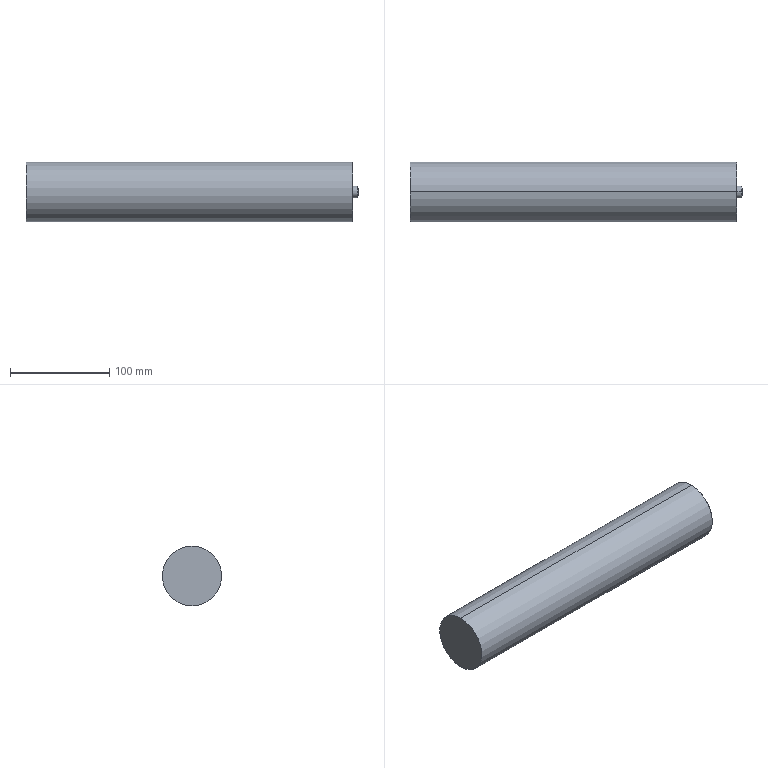Part | STEP file | Unpowered roller | 1 solid | 18 faces | box 334.5 x 60 x 60 mm | volume 930239 mm3 | cone 8 | cylinder 6 | plane 4 | commonest cylinder face diameters 6.8 x2 12 x2 60 x2
STEP:
#1=CARTESIAN_POINT('',(64.,0.,30.));
#2=VERTEX_POINT('',#1);
#3=CARTESIAN_POINT('',(64.,0.,-30.));
#4=VERTEX_POINT('',#3);
#5=CARTESIAN_POINT('',(64.,0.,0.));
#6=DIRECTION('',(-1.,0.,0.));
#7=DIRECTION('',(0.,0.,1.));
#8=AXIS2_PLACEMENT_3D('',#5,#6,#7);
#9=CIRCLE('',#8,30.);
#10=EDGE_CURVE('',#2,#4,#9,.T.);
#11=ORIENTED_EDGE('',*,*,#10,.T.);
#12=CARTESIAN_POINT('',(-264.5,0.,-30.));
#13=VERTEX_POINT('',#12);
#14=CARTESIAN_POINT('',(64.5,0.,-30.));
#15=DIRECTION('',(-1.,0.,0.));
#16=VECTOR('',#15,1000.);
#17=LINE('',#14,#16);
#18=EDGE_CURVE('',#4,#13,#17,.T.);
#19=ORIENTED_EDGE('',*,*,#18,.T.);
#20=CARTESIAN_POINT('',(-264.5,0.,30.));
#21=VERTEX_POINT('',#20);
#22=CARTESIAN_POINT('',(-264.5,0.,0.));
#23=DIRECTION('',(-1.,0.,0.));
#24=DIRECTION('',(0.,0.,1.));
#25=AXIS2_PLACEMENT_3D('',#22,#23,#24);
#26=CIRCLE('',#25,30.);
#27=EDGE_CURVE('',#21,#13,#26,.T.);
#28=ORIENTED_EDGE('',*,*,#27,.F.);
#29=CARTESIAN_POINT('',(64.5,0.,30.));
#30=DIRECTION('',(-1.,0.,0.));
#31=VECTOR('',#30,1000.);
#32=LINE('',#29,#31);
#33=EDGE_CURVE('',#2,#21,#32,.T.);
#34=ORIENTED_EDGE('',*,*,#33,.F.);
#35=EDGE_LOOP('',(#11,#19,#28,#34));
#36=FACE_OUTER_BOUND('',#35,.T.);
#37=CARTESIAN_POINT('',(64.5,0.,0.));
#38=DIRECTION('',(-1.,0.,0.));
#39=DIRECTION('',(0.,0.,1.));
#40=AXIS2_PLACEMENT_3D('',#37,#38,#39);
#41=CYLINDRICAL_SURFACE('',#40,30.);
#42=ADVANCED_FACE('',(#36),#41,.T.);
#43=CARTESIAN_POINT('',(64.5,0.,29.5));
#44=VERTEX_POINT('',#43);
#45=CARTESIAN_POINT('',(64.5,0.,-29.5));
#46=VERTEX_POINT('',#45);
#47=CARTESIAN_POINT('',(64.5,0.,0.));
#48=DIRECTION('',(-1.,0.,0.));
#49=DIRECTION('',(0.,0.,1.));
#50=AXIS2_PLACEMENT_3D('',#47,#48,#49);
#51=CIRCLE('',#50,29.5);
#52=EDGE_CURVE('',#44,#46,#51,.T.);
#53=ORIENTED_EDGE('',*,*,#52,.T.);
#54=CARTESIAN_POINT('',(64.,0.,-30.));
#55=DIRECTION('',(-0.7071,0.,-0.7071));
#56=VECTOR('',#55,1000.);
#57=LINE('',#54,#56);
#58=EDGE_CURVE('',#46,#4,#57,.T.);
#59=ORIENTED_EDGE('',*,*,#58,.T.);
#60=ORIENTED_EDGE('',*,*,#10,.F.);
#61=CARTESIAN_POINT('',(64.,0.,30.));
#62=DIRECTION('',(-0.7071,0.,0.7071));
#63=VECTOR('',#62,1000.);
#64=LINE('',#61,#63);
#65=EDGE_CURVE('',#44,#2,#64,.T.);
#66=ORIENTED_EDGE('',*,*,#65,.F.);
#67=EDGE_LOOP('',(#53,#59,#60,#66));
#68=FACE_OUTER_BOUND('',#67,.T.);
#69=CARTESIAN_POINT('',(64.,0.,0.));
#70=DIRECTION('',(-1.,0.,0.));
#71=DIRECTION('',(0.,0.,1.));
#72=AXIS2_PLACEMENT_3D('',#69,#70,#71);
#73=CONICAL_SURFACE('',#72,30.,0.7854);
#74=ADVANCED_FACE('',(#68),#73,.T.);
#75=CARTESIAN_POINT('',(69.5,0.,6.));
#76=VERTEX_POINT('',#75);
#77=CARTESIAN_POINT('',(69.5,0.,-6.));
#78=VERTEX_POINT('',#77);
#79=CARTESIAN_POINT('',(69.5,0.,0.));
#80=DIRECTION('',(-1.,0.,0.));
#81=DIRECTION('',(0.,0.,1.));
#82=AXIS2_PLACEMENT_3D('',#79,#80,#81);
#83=CIRCLE('',#82,6.);
#84=EDGE_CURVE('',#76,#78,#83,.T.);
#85=ORIENTED_EDGE('',*,*,#84,.T.);
#86=CARTESIAN_POINT('',(64.5,0.,-6.));
#87=VERTEX_POINT('',#86);
#88=CARTESIAN_POINT('',(70.,0.,-6.));
#89=DIRECTION('',(-1.,0.,0.));
#90=VECTOR('',#89,1000.);
#91=LINE('',#88,#90);
#92=EDGE_CURVE('',#78,#87,#91,.T.);
#93=ORIENTED_EDGE('',*,*,#92,.T.);
#94=CARTESIAN_POINT('',(64.5,0.,6.));
#95=VERTEX_POINT('',#94);
#96=CARTESIAN_POINT('',(64.5,0.,0.));
#97=DIRECTION('',(-1.,0.,0.));
#98=DIRECTION('',(0.,0.,1.));
#99=AXIS2_PLACEMENT_3D('',#96,#97,#98);
#100=CIRCLE('',#99,6.);
#101=EDGE_CURVE('',#95,#87,#100,.T.);
#102=ORIENTED_EDGE('',*,*,#101,.F.);
#103=CARTESIAN_POINT('',(70.,0.,6.));
#104=DIRECTION('',(-1.,0.,0.));
#105=VECTOR('',#104,1000.);
#106=LINE('',#103,#105);
#107=EDGE_CURVE('',#76,#95,#106,.T.);
#108=ORIENTED_EDGE('',*,*,#107,.F.);
#109=EDGE_LOOP('',(#85,#93,#102,#108));
#110=FACE_OUTER_BOUND('',#109,.T.);
#111=CARTESIAN_POINT('',(70.,0.,0.));
#112=DIRECTION('',(-1.,0.,0.));
#113=DIRECTION('',(0.,0.,1.));
#114=AXIS2_PLACEMENT_3D('',#111,#112,#113);
#115=CYLINDRICAL_SURFACE('',#114,6.);
#116=ADVANCED_FACE('',(#110),#115,.T.);
#117=CARTESIAN_POINT('',(70.,0.,5.5));
#118=VERTEX_POINT('',#117);
#119=CARTESIAN_POINT('',(70.,0.,-5.5));
#120=VERTEX_POINT('',#119);
#121=CARTESIAN_POINT('',(70.,0.,0.));
#122=DIRECTION('',(-1.,0.,0.));
#123=DIRECTION('',(0.,0.,1.));
#124=AXIS2_PLACEMENT_3D('',#121,#122,#123);
#125=CIRCLE('',#124,5.5);
#126=EDGE_CURVE('',#118,#120,#125,.T.);
#127=ORIENTED_EDGE('',*,*,#126,.T.);
#128=CARTESIAN_POINT('',(69.5,0.,-6.));
#129=DIRECTION('',(-0.7071,0.,-0.7071));
#130=VECTOR('',#129,1000.);
#131=LINE('',#128,#130);
#132=EDGE_CURVE('',#120,#78,#131,.T.);
#133=ORIENTED_EDGE('',*,*,#132,.T.);
#134=ORIENTED_EDGE('',*,*,#84,.F.);
#135=CARTESIAN_POINT('',(69.5,0.,6.));
#136=DIRECTION('',(-0.7071,0.,0.7071));
#137=VECTOR('',#136,1000.);
#138=LINE('',#135,#137);
#139=EDGE_CURVE('',#118,#76,#138,.T.);
#140=ORIENTED_EDGE('',*,*,#139,.F.);
#141=EDGE_LOOP('',(#127,#133,#134,#140));
#142=FACE_OUTER_BOUND('',#141,.T.);
#143=CARTESIAN_POINT('',(69.5,0.,0.));
#144=DIRECTION('',(-1.,0.,0.));
#145=DIRECTION('',(0.,0.,1.));
#146=AXIS2_PLACEMENT_3D('',#143,#144,#145);
#147=CONICAL_SURFACE('',#146,6.,0.7854);
#148=ADVANCED_FACE('',(#142),#147,.T.);
#149=CARTESIAN_POINT('',(55.,0.,3.4));
#150=VERTEX_POINT('',#149);
#151=CARTESIAN_POINT('',(55.,0.,-3.4));
#152=VERTEX_POINT('',#151);
#153=CARTESIAN_POINT('',(55.,0.,0.));
#154=DIRECTION('',(1.,0.,0.));
#155=DIRECTION('',(0.,0.,-1.));
#156=AXIS2_PLACEMENT_3D('',#153,#154,#155);
#157=CIRCLE('',#156,3.4);
#158=EDGE_CURVE('',#150,#152,#157,.T.);
#159=ORIENTED_EDGE('',*,*,#158,.F.);
#160=CARTESIAN_POINT('',(70.,0.,3.4));
#161=VERTEX_POINT('',#160);
#162=CARTESIAN_POINT('',(70.,0.,3.4));
#163=DIRECTION('',(1.,0.,0.));
#164=VECTOR('',#163,1000.);
#165=LINE('',#162,#164);
#166=EDGE_CURVE('',#150,#161,#165,.T.);
#167=ORIENTED_EDGE('',*,*,#166,.T.);
#168=CARTESIAN_POINT('',(70.,0.,-3.4));
#169=VERTEX_POINT('',#168);
#170=CARTESIAN_POINT('',(70.,0.,0.));
#171=DIRECTION('',(-1.,0.,0.));
#172=DIRECTION('',(0.,0.,-1.));
#173=AXIS2_PLACEMENT_3D('',#170,#171,#172);
#174=CIRCLE('',#173,3.4);
#175=EDGE_CURVE('',#169,#161,#174,.T.);
#176=ORIENTED_EDGE('',*,*,#175,.F.);
#177=CARTESIAN_POINT('',(70.,0.,-3.4));
#178=DIRECTION('',(1.,0.,0.));
#179=VECTOR('',#178,1000.);
#180=LINE('',#177,#179);
#181=EDGE_CURVE('',#152,#169,#180,.T.);
#182=ORIENTED_EDGE('',*,*,#181,.F.);
#183=EDGE_LOOP('',(#159,#167,#176,#182));
#184=FACE_OUTER_BOUND('',#183,.T.);
#185=CARTESIAN_POINT('',(70.,0.,0.));
#186=DIRECTION('',(1.,0.,0.));
#187=DIRECTION('',(0.,0.,-1.));
#188=AXIS2_PLACEMENT_3D('',#185,#186,#187);
#189=CYLINDRICAL_SURFACE('',#188,3.4);
#190=ADVANCED_FACE('',(#184),#189,.F.);
#191=CARTESIAN_POINT('',(52.957,0.,0.));
#192=VERTEX_POINT('',#191);
#193=CARTESIAN_POINT('',(55.,0.,-3.4));
#194=DIRECTION('',(0.515,0.,-0.8572));
#195=VECTOR('',#194,1000.);
#196=LINE('',#193,#195);
#197=EDGE_CURVE('',#192,#152,#196,.T.);
#198=ORIENTED_EDGE('',*,*,#197,.F.);
#199=CARTESIAN_POINT('',(55.,0.,3.4));
#200=DIRECTION('',(0.515,0.,0.8572));
#201=VECTOR('',#200,1000.);
#202=LINE('',#199,#201);
#203=EDGE_CURVE('',#192,#150,#202,.T.);
#204=ORIENTED_EDGE('',*,*,#203,.T.);
#205=ORIENTED_EDGE('',*,*,#158,.T.);
#206=EDGE_LOOP('',(#198,#204,#205));
#207=FACE_OUTER_BOUND('',#206,.T.);
#208=CARTESIAN_POINT('',(55.,0.,0.));
#209=DIRECTION('',(1.,0.,0.));
#210=DIRECTION('',(0.,0.,-1.));
#211=AXIS2_PLACEMENT_3D('',#208,#209,#210);
#212=CONICAL_SURFACE('',#211,3.4,1.03);
#213=ADVANCED_FACE('',(#207),#212,.F.);
#214=ORIENTED_EDGE('',*,*,#203,.F.);
#215=ORIENTED_EDGE('',*,*,#197,.T.);
#216=CARTESIAN_POINT('',(55.,0.,0.));
#217=DIRECTION('',(1.,0.,0.));
#218=DIRECTION('',(0.,0.,-1.));
#219=AXIS2_PLACEMENT_3D('',#216,#217,#218);
#220=CIRCLE('',#219,3.4);
#221=EDGE_CURVE('',#152,#150,#220,.T.);
#222=ORIENTED_EDGE('',*,*,#221,.T.);
#223=EDGE_LOOP('',(#214,#215,#222));
#224=FACE_OUTER_BOUND('',#223,.T.);
#225=CARTESIAN_POINT('',(55.,0.,0.));
#226=DIRECTION('',(1.,0.,0.));
#227=DIRECTION('',(0.,0.,-1.));
#228=AXIS2_PLACEMENT_3D('',#225,#226,#227);
#229=CONICAL_SURFACE('',#228,3.4,1.03);
#230=ADVANCED_FACE('',(#224),#229,.F.);
#231=ORIENTED_EDGE('',*,*,#166,.F.);
#232=ORIENTED_EDGE('',*,*,#221,.F.);
#233=ORIENTED_EDGE('',*,*,#181,.T.);
#234=CARTESIAN_POINT('',(70.,0.,0.));
#235=DIRECTION('',(-1.,0.,0.));
#236=DIRECTION('',(0.,0.,-1.));
#237=AXIS2_PLACEMENT_3D('',#234,#235,#236);
#238=CIRCLE('',#237,3.4);
#239=EDGE_CURVE('',#161,#169,#238,.T.);
#240=ORIENTED_EDGE('',*,*,#239,.F.);
#241=EDGE_LOOP('',(#231,#232,#233,#240));
#242=FACE_OUTER_BOUND('',#241,.T.);
#243=CARTESIAN_POINT('',(70.,0.,0.));
#244=DIRECTION('',(1.,0.,0.));
#245=DIRECTION('',(0.,0.,-1.));
#246=AXIS2_PLACEMENT_3D('',#243,#244,#245);
#247=CYLINDRICAL_SURFACE('',#246,3.4);
#248=ADVANCED_FACE('',(#242),#247,.F.);
#249=ORIENTED_EDGE('',*,*,#126,.F.);
#250=CARTESIAN_POINT('',(70.,0.,0.));
#251=DIRECTION('',(-1.,0.,0.));
#252=DIRECTION('',(0.,0.,1.));
#253=AXIS2_PLACEMENT_3D('',#250,#251,#252);
#254=CIRCLE('',#253,5.5);
#255=EDGE_CURVE('',#120,#118,#254,.T.);
#256=ORIENTED_EDGE('',*,*,#255,.F.);
#257=EDGE_LOOP('',(#249,#256));
#258=FACE_OUTER_BOUND('',#257,.T.);
#259=ORIENTED_EDGE('',*,*,#175,.T.);
#260=ORIENTED_EDGE('',*,*,#239,.T.);
#261=EDGE_LOOP('',(#259,#260));
#262=FACE_BOUND('',#261,.T.);
#263=CARTESIAN_POINT('',(70.,0.,0.));
#264=DIRECTION('',(1.,0.,0.));
#265=DIRECTION('',(0.,0.,-1.));
#266=AXIS2_PLACEMENT_3D('',#263,#264,#265);
#267=PLANE('',#266);
#268=ADVANCED_FACE('',(#258,#262),#267,.T.);
#269=ORIENTED_EDGE('',*,*,#132,.F.);
#270=ORIENTED_EDGE('',*,*,#255,.T.);
#271=ORIENTED_EDGE('',*,*,#139,.T.);
#272=CARTESIAN_POINT('',(69.5,0.,0.));
#273=DIRECTION('',(-1.,0.,0.));
#274=DIRECTION('',(0.,0.,1.));
#275=AXIS2_PLACEMENT_3D('',#272,#273,#274);
#276=CIRCLE('',#275,6.);
#277=EDGE_CURVE('',#78,#76,#276,.T.);
#278=ORIENTED_EDGE('',*,*,#277,.F.);
#279=EDGE_LOOP('',(#269,#270,#271,#278));
#280=FACE_OUTER_BOUND('',#279,.T.);
#281=CARTESIAN_POINT('',(69.5,0.,0.));
#282=DIRECTION('',(-1.,0.,0.));
#283=DIRECTION('',(0.,0.,1.));
#284=AXIS2_PLACEMENT_3D('',#281,#282,#283);
#285=CONICAL_SURFACE('',#284,6.,0.7854);
#286=ADVANCED_FACE('',(#280),#285,.T.);
#287=ORIENTED_EDGE('',*,*,#92,.F.);
#288=ORIENTED_EDGE('',*,*,#277,.T.);
#289=ORIENTED_EDGE('',*,*,#107,.T.);
#290=CARTESIAN_POINT('',(64.5,0.,0.));
#291=DIRECTION('',(-1.,0.,0.));
#292=DIRECTION('',(0.,0.,1.));
#293=AXIS2_PLACEMENT_3D('',#290,#291,#292);
#294=CIRCLE('',#293,6.);
#295=EDGE_CURVE('',#87,#95,#294,.T.);
#296=ORIENTED_EDGE('',*,*,#295,.F.);
#297=EDGE_LOOP('',(#287,#288,#289,#296));
#298=FACE_OUTER_BOUND('',#297,.T.);
#299=CARTESIAN_POINT('',(70.,0.,0.));
#300=DIRECTION('',(-1.,0.,0.));
#301=DIRECTION('',(0.,0.,1.));
#302=AXIS2_PLACEMENT_3D('',#299,#300,#301);
#303=CYLINDRICAL_SURFACE('',#302,6.);
#304=ADVANCED_FACE('',(#298),#303,.T.);
#305=ORIENTED_EDGE('',*,*,#101,.T.);
#306=ORIENTED_EDGE('',*,*,#295,.T.);
#307=EDGE_LOOP('',(#305,#306));
#308=FACE_BOUND('',#307,.T.);
#309=ORIENTED_EDGE('',*,*,#52,.F.);
#310=CARTESIAN_POINT('',(64.5,0.,0.));
#311=DIRECTION('',(-1.,0.,0.));
#312=DIRECTION('',(0.,0.,1.));
#313=AXIS2_PLACEMENT_3D('',#310,#311,#312);
#314=CIRCLE('',#313,29.5);
#315=EDGE_CURVE('',#46,#44,#314,.T.);
#316=ORIENTED_EDGE('',*,*,#315,.F.);
#317=EDGE_LOOP('',(#309,#316));
#318=FACE_OUTER_BOUND('',#317,.T.);
#319=CARTESIAN_POINT('',(64.5,0.,0.));
#320=DIRECTION('',(1.,0.,0.));
#321=DIRECTION('',(0.,0.,-1.));
#322=AXIS2_PLACEMENT_3D('',#319,#320,#321);
#323=PLANE('',#322);
#324=ADVANCED_FACE('',(#308,#318),#323,.T.);
#325=ORIENTED_EDGE('',*,*,#58,.F.);
#326=ORIENTED_EDGE('',*,*,#315,.T.);
#327=ORIENTED_EDGE('',*,*,#65,.T.);
#328=CARTESIAN_POINT('',(64.,0.,0.));
#329=DIRECTION('',(-1.,0.,0.));
#330=DIRECTION('',(0.,0.,1.));
#331=AXIS2_PLACEMENT_3D('',#328,#329,#330);
#332=CIRCLE('',#331,30.);
#333=EDGE_CURVE('',#4,#2,#332,.T.);
#334=ORIENTED_EDGE('',*,*,#333,.F.);
#335=EDGE_LOOP('',(#325,#326,#327,#334));
#336=FACE_OUTER_BOUND('',#335,.T.);
#337=CARTESIAN_POINT('',(64.,0.,0.));
#338=DIRECTION('',(-1.,0.,0.));
#339=DIRECTION('',(0.,0.,1.));
#340=AXIS2_PLACEMENT_3D('',#337,#338,#339);
#341=CONICAL_SURFACE('',#340,30.,0.7854);
#342=ADVANCED_FACE('',(#336),#341,.T.);
#343=ORIENTED_EDGE('',*,*,#18,.F.);
#344=ORIENTED_EDGE('',*,*,#333,.T.);
#345=ORIENTED_EDGE('',*,*,#33,.T.);
#346=CARTESIAN_POINT('',(-264.5,0.,0.));
#347=DIRECTION('',(-1.,0.,0.));
#348=DIRECTION('',(0.,0.,1.));
#349=AXIS2_PLACEMENT_3D('',#346,#347,#348);
#350=CIRCLE('',#349,30.);
#351=EDGE_CURVE('',#13,#21,#350,.T.);
#352=ORIENTED_EDGE('',*,*,#351,.F.);
#353=EDGE_LOOP('',(#343,#344,#345,#352));
#354=FACE_OUTER_BOUND('',#353,.T.);
#355=CARTESIAN_POINT('',(64.5,0.,0.));
#356=DIRECTION('',(-1.,0.,0.));
#357=DIRECTION('',(0.,0.,1.));
#358=AXIS2_PLACEMENT_3D('',#355,#356,#357);
#359=CYLINDRICAL_SURFACE('',#358,30.);
#360=ADVANCED_FACE('',(#354),#359,.T.);
#361=ORIENTED_EDGE('',*,*,#27,.T.);
#362=ORIENTED_EDGE('',*,*,#351,.T.);
#363=EDGE_LOOP('',(#361,#362));
#364=FACE_OUTER_BOUND('',#363,.T.);
#365=CARTESIAN_POINT('',(-264.5,0.,0.));
#366=DIRECTION('',(-1.,0.,0.));
#367=DIRECTION('',(0.,0.,1.));
#368=AXIS2_PLACEMENT_3D('',#365,#366,#367);
#369=PLANE('',#368);
#370=ADVANCED_FACE('',(#364),#369,.T.);
#371=CLOSED_SHELL('',(#42,#74,#116,#148,#190,#213,#230,#248,#268,#286,#304,#324,#342,#360,#370));
#372=CARTESIAN_POINT('',(-52.957,0.,0.));
#373=VERTEX_POINT('',#372);
#374=CARTESIAN_POINT('',(-54.5,0.,2.568));
#375=VERTEX_POINT('',#374);
#376=CARTESIAN_POINT('',(-55.,0.,3.4));
#377=DIRECTION('',(-0.515,0.,0.8572));
#378=VECTOR('',#377,1000.);
#379=LINE('',#376,#378);
#380=EDGE_CURVE('',#373,#375,#379,.T.);
#381=ORIENTED_EDGE('',*,*,#380,.F.);
#382=CARTESIAN_POINT('',(-54.5,0.,-2.568));
#383=VERTEX_POINT('',#382);
#384=CARTESIAN_POINT('',(-55.,0.,-3.4));
#385=DIRECTION('',(-0.515,0.,-0.8572));
#386=VECTOR('',#385,1000.);
#387=LINE('',#384,#386);
#388=EDGE_CURVE('',#373,#383,#387,.T.);
#389=ORIENTED_EDGE('',*,*,#388,.T.);
#390=CARTESIAN_POINT('',(-54.5,0.,0.));
#391=DIRECTION('',(1.,0.,0.));
#392=DIRECTION('',(0.,0.,1.));
#393=AXIS2_PLACEMENT_3D('',#390,#391,#392);
#394=CIRCLE('',#393,2.568);
#395=EDGE_CURVE('',#375,#383,#394,.T.);
#396=ORIENTED_EDGE('',*,*,#395,.F.);
#397=EDGE_LOOP('',(#381,#389,#396));
#398=FACE_OUTER_BOUND('',#397,.T.);
#399=CARTESIAN_POINT('',(-55.,0.,0.));
#400=DIRECTION('',(-1.,0.,0.));
#401=DIRECTION('',(0.,0.,1.));
#402=AXIS2_PLACEMENT_3D('',#399,#400,#401);
#403=CONICAL_SURFACE('',#402,3.4,1.03);
#404=ADVANCED_FACE('',(#398),#403,.F.);
#405=ORIENTED_EDGE('',*,*,#395,.T.);
#406=CARTESIAN_POINT('',(-54.5,0.,0.));
#407=DIRECTION('',(1.,0.,0.));
#408=DIRECTION('',(0.,0.,1.));
#409=AXIS2_PLACEMENT_3D('',#406,#407,#408);
#410=CIRCLE('',#409,2.568);
#411=EDGE_CURVE('',#383,#375,#410,.T.);
#412=ORIENTED_EDGE('',*,*,#411,.T.);
#413=EDGE_LOOP('',(#405,#412));
#414=FACE_OUTER_BOUND('',#413,.T.);
#415=CARTESIAN_POINT('',(-54.5,0.,0.));
#416=DIRECTION('',(-1.,0.,0.));
#417=DIRECTION('',(0.,0.,1.));
#418=AXIS2_PLACEMENT_3D('',#415,#416,#417);
#419=PLANE('',#418);
#420=ADVANCED_FACE('',(#414),#419,.F.);
#421=ORIENTED_EDGE('',*,*,#388,.F.);
#422=ORIENTED_EDGE('',*,*,#380,.T.);
#423=ORIENTED_EDGE('',*,*,#411,.F.);
#424=EDGE_LOOP('',(#421,#422,#423));
#425=FACE_OUTER_BOUND('',#424,.T.);
#426=CARTESIAN_POINT('',(-55.,0.,0.));
#427=DIRECTION('',(-1.,0.,0.));
#428=DIRECTION('',(0.,0.,1.));
#429=AXIS2_PLACEMENT_3D('',#426,#427,#428);
#430=CONICAL_SURFACE('',#429,3.4,1.03);
#431=ADVANCED_FACE('',(#425),#430,.F.);
#432=CLOSED_SHELL('',(#404,#420,#431));
#433=ORIENTED_CLOSED_SHELL('',*,#432,.F.);
#434=BREP_WITH_VOIDS('',#371,(#433));
#435=CARTESIAN_POINT('',(0.,0.,0.));
#436=DIRECTION('',(0.,0.,1.));
#437=DIRECTION('',(1.,0.,0.));
#438=AXIS2_PLACEMENT_3D('',#435,#436,#437);
#439=(LENGTH_UNIT()NAMED_UNIT(*)SI_UNIT(.MILLI.,.METRE.));
#440=UNCERTAINTY_MEASURE_WITH_UNIT(LENGTH_MEASURE(0.00001),#439,'','');
#441=(NAMED_UNIT(*)PLANE_ANGLE_UNIT()SI_UNIT($,.RADIAN.));
#442=(NAMED_UNIT(*)SI_UNIT($,.STERADIAN.)SOLID_ANGLE_UNIT());
#443=(GEOMETRIC_REPRESENTATION_CONTEXT(3)GLOBAL_UNCERTAINTY_ASSIGNED_CONTEXT((#440))GLOBAL_UNIT_ASSIGNED_CONTEXT((#439,#441,#442))REPRESENTATION_CONTEXT('',''));
#444=ADVANCED_BREP_SHAPE_REPRESENTATION('',(#434,#438),#443);